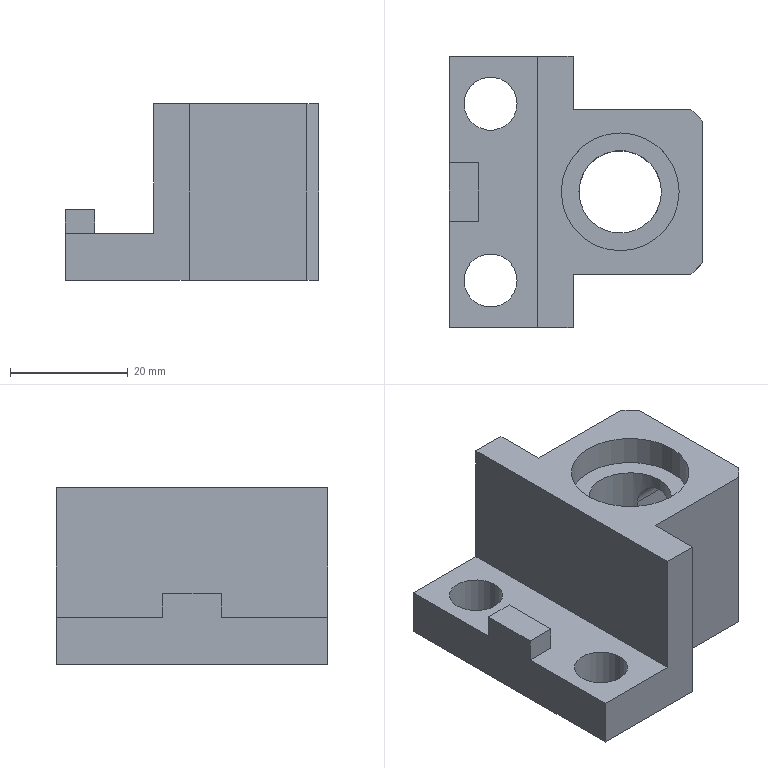Part | SolidWorks | features ICE 4, Chamfer 1, Extrusion 1 | 1 solid | 32 faces | box 43 x 46 x 30 mm | volume 25082 mm3 | plane 21 | cylinder 11 | commonest cylinder face diameters 9 x4 8 x3 14 x2 20 x2
STEP:
#1=CARTESIAN_POINT('',(13.245,4.,11.));
#2=VERTEX_POINT('',#1);
#3=CARTESIAN_POINT('',(14.5,0.,7.));
#4=VERTEX_POINT('',#3);
#5=CARTESIAN_POINT('',(13.245,4.,11.));
#6=CARTESIAN_POINT('',(13.245,4.,10.729));
#7=CARTESIAN_POINT('',(13.264,3.973,10.464));
#8=CARTESIAN_POINT('',(13.335,3.867,9.944));
#9=CARTESIAN_POINT('',(13.388,3.788,9.688));
#10=CARTESIAN_POINT('',(13.576,3.484,8.968));
#11=CARTESIAN_POINT('',(13.743,3.191,8.535));
#12=CARTESIAN_POINT('',(13.982,2.65,7.993));
#13=CARTESIAN_POINT('',(14.061,2.449,7.827));
#14=CARTESIAN_POINT('',(14.206,2.021,7.538));
#15=CARTESIAN_POINT('',(14.271,1.794,7.415));
#16=CARTESIAN_POINT('',(14.38,1.312,7.212));
#17=CARTESIAN_POINT('',(14.425,1.054,7.132));
#18=CARTESIAN_POINT('',(14.485,0.5336,7.027));
#19=CARTESIAN_POINT('',(14.5,0.269,7.));
#20=CARTESIAN_POINT('',(14.5,0.,7.));
#21=B_SPLINE_CURVE_WITH_KNOTS('',3,(#5,#6,#7,#8,#9,#10,#11,#12,#13,#14,#15,#16,#17,#18,#19,#20),.UNSPECIFIED.,.F.,.F.,(4,2,2,2,2,2,2,4),(0.,0.0008004,0.001601,0.003201,0.004002,0.004802,0.005603,0.006403),.UNSPECIFIED.);
#22=EDGE_CURVE('',#2,#4,#21,.T.);
#23=ORIENTED_EDGE('',*,*,#22,.T.);
#24=CARTESIAN_POINT('',(21.5,0.,7.));
#25=VERTEX_POINT('',#24);
#26=CARTESIAN_POINT('',(9.5,0.,7.));
#27=DIRECTION('',(1.,0.,0.));
#28=VECTOR('',#27,1000.);
#29=LINE('',#26,#28);
#30=EDGE_CURVE('',#4,#25,#29,.T.);
#31=ORIENTED_EDGE('',*,*,#30,.T.);
#32=CARTESIAN_POINT('',(21.5,4.,11.));
#33=VERTEX_POINT('',#32);
#34=CARTESIAN_POINT('',(21.5,0.,11.));
#35=DIRECTION('',(1.,0.,0.));
#36=DIRECTION('',(0.,0.,1.));
#37=AXIS2_PLACEMENT_3D('',#34,#35,#36);
#38=CIRCLE('',#37,4.);
#39=EDGE_CURVE('',#25,#33,#38,.T.);
#40=ORIENTED_EDGE('',*,*,#39,.T.);
#41=CARTESIAN_POINT('',(9.5,4.,11.));
#42=DIRECTION('',(1.,0.,0.));
#43=VECTOR('',#42,1000.);
#44=LINE('',#41,#43);
#45=EDGE_CURVE('',#2,#33,#44,.T.);
#46=ORIENTED_EDGE('',*,*,#45,.F.);
#47=EDGE_LOOP('',(#23,#31,#40,#46));
#48=FACE_OUTER_BOUND('',#47,.T.);
#49=CARTESIAN_POINT('',(9.5,0.,11.));
#50=DIRECTION('',(1.,0.,0.));
#51=DIRECTION('',(0.,0.,-1.));
#52=AXIS2_PLACEMENT_3D('',#49,#50,#51);
#53=CYLINDRICAL_SURFACE('',#52,4.);
#54=ADVANCED_FACE('',(#48),#53,.F.);
#55=CARTESIAN_POINT('',(-2.5,0.,25.));
#56=VERTEX_POINT('',#55);
#57=CARTESIAN_POINT('',(17.5,0.,25.));
#58=VERTEX_POINT('',#57);
#59=CARTESIAN_POINT('',(7.5,0.,25.));
#60=DIRECTION('',(0.,0.,1.));
#61=DIRECTION('',(1.,0.,0.));
#62=AXIS2_PLACEMENT_3D('',#59,#60,#61);
#63=CIRCLE('',#62,10.);
#64=EDGE_CURVE('',#56,#58,#63,.T.);
#65=ORIENTED_EDGE('',*,*,#64,.F.);
#66=CARTESIAN_POINT('',(-2.5,0.,30.));
#67=VERTEX_POINT('',#66);
#68=CARTESIAN_POINT('',(-2.5,0.,25.));
#69=DIRECTION('',(0.,0.,1.));
#70=VECTOR('',#69,1000.);
#71=LINE('',#68,#70);
#72=EDGE_CURVE('',#56,#67,#71,.T.);
#73=ORIENTED_EDGE('',*,*,#72,.T.);
#74=CARTESIAN_POINT('',(17.5,0.,30.));
#75=VERTEX_POINT('',#74);
#76=CARTESIAN_POINT('',(7.5,0.,30.));
#77=DIRECTION('',(0.,0.,1.));
#78=DIRECTION('',(1.,0.,0.));
#79=AXIS2_PLACEMENT_3D('',#76,#77,#78);
#80=CIRCLE('',#79,10.);
#81=EDGE_CURVE('',#67,#75,#80,.T.);
#82=ORIENTED_EDGE('',*,*,#81,.T.);
#83=CARTESIAN_POINT('',(17.5,0.,25.));
#84=DIRECTION('',(0.,0.,1.));
#85=VECTOR('',#84,1000.);
#86=LINE('',#83,#85);
#87=EDGE_CURVE('',#58,#75,#86,.T.);
#88=ORIENTED_EDGE('',*,*,#87,.F.);
#89=EDGE_LOOP('',(#65,#73,#82,#88));
#90=FACE_OUTER_BOUND('',#89,.T.);
#91=CARTESIAN_POINT('',(7.5,0.,25.));
#92=DIRECTION('',(0.,0.,1.));
#93=DIRECTION('',(1.,0.,0.));
#94=AXIS2_PLACEMENT_3D('',#91,#92,#93);
#95=CYLINDRICAL_SURFACE('',#94,10.);
#96=ADVANCED_FACE('',(#90),#95,.F.);
#97=CARTESIAN_POINT('',(-10.,-15.,8.));
#98=VERTEX_POINT('',#97);
#99=CARTESIAN_POINT('',(-19.,-15.,8.));
#100=VERTEX_POINT('',#99);
#101=CARTESIAN_POINT('',(-14.5,-15.,8.));
#102=DIRECTION('',(0.,0.,-1.));
#103=DIRECTION('',(-1.,0.,0.));
#104=AXIS2_PLACEMENT_3D('',#101,#102,#103);
#105=CIRCLE('',#104,4.5);
#106=EDGE_CURVE('',#98,#100,#105,.T.);
#107=ORIENTED_EDGE('',*,*,#106,.F.);
#108=CARTESIAN_POINT('',(-10.,-15.,0.));
#109=VERTEX_POINT('',#108);
#110=CARTESIAN_POINT('',(-10.,-15.,30.));
#111=DIRECTION('',(0.,0.,-1.));
#112=VECTOR('',#111,1000.);
#113=LINE('',#110,#112);
#114=EDGE_CURVE('',#98,#109,#113,.T.);
#115=ORIENTED_EDGE('',*,*,#114,.T.);
#116=CARTESIAN_POINT('',(-19.,-15.,0.));
#117=VERTEX_POINT('',#116);
#118=CARTESIAN_POINT('',(-14.5,-15.,0.));
#119=DIRECTION('',(0.,0.,1.));
#120=DIRECTION('',(1.,0.,0.));
#121=AXIS2_PLACEMENT_3D('',#118,#119,#120);
#122=CIRCLE('',#121,4.5);
#123=EDGE_CURVE('',#117,#109,#122,.T.);
#124=ORIENTED_EDGE('',*,*,#123,.F.);
#125=CARTESIAN_POINT('',(-19.,-15.,30.));
#126=DIRECTION('',(0.,0.,-1.));
#127=VECTOR('',#126,1000.);
#128=LINE('',#125,#127);
#129=EDGE_CURVE('',#100,#117,#128,.T.);
#130=ORIENTED_EDGE('',*,*,#129,.F.);
#131=EDGE_LOOP('',(#107,#115,#124,#130));
#132=FACE_OUTER_BOUND('',#131,.T.);
#133=CARTESIAN_POINT('',(-14.5,-15.,30.));
#134=DIRECTION('',(0.,0.,-1.));
#135=DIRECTION('',(-1.,0.,0.));
#136=AXIS2_PLACEMENT_3D('',#133,#134,#135);
#137=CYLINDRICAL_SURFACE('',#136,4.5);
#138=ADVANCED_FACE('',(#132),#137,.F.);
#139=CARTESIAN_POINT('',(-10.,15.,8.));
#140=VERTEX_POINT('',#139);
#141=CARTESIAN_POINT('',(-19.,15.,8.));
#142=VERTEX_POINT('',#141);
#143=CARTESIAN_POINT('',(-14.5,15.,8.));
#144=DIRECTION('',(0.,0.,-1.));
#145=DIRECTION('',(-1.,0.,0.));
#146=AXIS2_PLACEMENT_3D('',#143,#144,#145);
#147=CIRCLE('',#146,4.5);
#148=EDGE_CURVE('',#140,#142,#147,.T.);
#149=ORIENTED_EDGE('',*,*,#148,.F.);
#150=CARTESIAN_POINT('',(-10.,15.,0.));
#151=VERTEX_POINT('',#150);
#152=CARTESIAN_POINT('',(-10.,15.,30.));
#153=DIRECTION('',(0.,0.,-1.));
#154=VECTOR('',#153,1000.);
#155=LINE('',#152,#154);
#156=EDGE_CURVE('',#140,#151,#155,.T.);
#157=ORIENTED_EDGE('',*,*,#156,.T.);
#158=CARTESIAN_POINT('',(-19.,15.,0.));
#159=VERTEX_POINT('',#158);
#160=CARTESIAN_POINT('',(-14.5,15.,0.));
#161=DIRECTION('',(0.,0.,1.));
#162=DIRECTION('',(1.,0.,0.));
#163=AXIS2_PLACEMENT_3D('',#160,#161,#162);
#164=CIRCLE('',#163,4.5);
#165=EDGE_CURVE('',#159,#151,#164,.T.);
#166=ORIENTED_EDGE('',*,*,#165,.F.);
#167=CARTESIAN_POINT('',(-19.,15.,30.));
#168=DIRECTION('',(0.,0.,-1.));
#169=VECTOR('',#168,1000.);
#170=LINE('',#167,#169);
#171=EDGE_CURVE('',#142,#159,#170,.T.);
#172=ORIENTED_EDGE('',*,*,#171,.F.);
#173=EDGE_LOOP('',(#149,#157,#166,#172));
#174=FACE_OUTER_BOUND('',#173,.T.);
#175=CARTESIAN_POINT('',(-14.5,15.,30.));
#176=DIRECTION('',(0.,0.,-1.));
#177=DIRECTION('',(-1.,0.,0.));
#178=AXIS2_PLACEMENT_3D('',#175,#176,#177);
#179=CYLINDRICAL_SURFACE('',#178,4.5);
#180=ADVANCED_FACE('',(#174),#179,.F.);
#181=CARTESIAN_POINT('',(0.5,0.,25.));
#182=VERTEX_POINT('',#181);
#183=CARTESIAN_POINT('',(14.5,0.,25.));
#184=VERTEX_POINT('',#183);
#185=CARTESIAN_POINT('',(7.5,0.,25.));
#186=DIRECTION('',(0.,0.,1.));
#187=DIRECTION('',(1.,0.,0.));
#188=AXIS2_PLACEMENT_3D('',#185,#186,#187);
#189=CIRCLE('',#188,7.);
#190=EDGE_CURVE('',#182,#184,#189,.T.);
#191=ORIENTED_EDGE('',*,*,#190,.T.);
#192=CARTESIAN_POINT('',(14.5,0.,23.));
#193=VERTEX_POINT('',#192);
#194=CARTESIAN_POINT('',(14.5,0.,30.));
#195=DIRECTION('',(0.,0.,-1.));
#196=VECTOR('',#195,1000.);
#197=LINE('',#194,#196);
#198=EDGE_CURVE('',#184,#193,#197,.T.);
#199=ORIENTED_EDGE('',*,*,#198,.T.);
#200=CARTESIAN_POINT('',(13.245,-4.,19.));
#201=VERTEX_POINT('',#200);
#202=CARTESIAN_POINT('',(13.245,-4.,19.));
#203=CARTESIAN_POINT('',(13.245,-4.,19.271));
#204=CARTESIAN_POINT('',(13.264,-3.973,19.536));
#205=CARTESIAN_POINT('',(13.335,-3.867,20.056));
#206=CARTESIAN_POINT('',(13.388,-3.788,20.312));
#207=CARTESIAN_POINT('',(13.576,-3.484,21.032));
#208=CARTESIAN_POINT('',(13.743,-3.191,21.465));
#209=CARTESIAN_POINT('',(13.982,-2.65,22.007));
#210=CARTESIAN_POINT('',(14.061,-2.449,22.173));
#211=CARTESIAN_POINT('',(14.206,-2.021,22.462));
#212=CARTESIAN_POINT('',(14.271,-1.794,22.585));
#213=CARTESIAN_POINT('',(14.38,-1.312,22.788));
#214=CARTESIAN_POINT('',(14.425,-1.054,22.868));
#215=CARTESIAN_POINT('',(14.485,-0.5336,22.973));
#216=CARTESIAN_POINT('',(14.5,-0.269,23.));
#217=CARTESIAN_POINT('',(14.5,0.,23.));
#218=B_SPLINE_CURVE_WITH_KNOTS('',3,(#202,#203,#204,#205,#206,#207,#208,#209,#210,#211,#212,#213,#214,#215,#216,#217),.UNSPECIFIED.,.F.,.F.,(4,2,2,2,2,2,2,4),(0.,0.0008004,0.001601,0.003201,0.004002,0.004802,0.005603,0.006403),.UNSPECIFIED.);
#219=EDGE_CURVE('',#201,#193,#218,.T.);
#220=ORIENTED_EDGE('',*,*,#219,.F.);
#221=CARTESIAN_POINT('',(13.245,-4.,11.));
#222=VERTEX_POINT('',#221);
#223=CARTESIAN_POINT('',(13.245,-4.,30.));
#224=DIRECTION('',(0.,0.,1.));
#225=VECTOR('',#224,1000.);
#226=LINE('',#223,#225);
#227=EDGE_CURVE('',#222,#201,#226,.T.);
#228=ORIENTED_EDGE('',*,*,#227,.F.);
#229=CARTESIAN_POINT('',(14.5,0.,7.));
#230=CARTESIAN_POINT('',(14.5,-0.1342,7.));
#231=CARTESIAN_POINT('',(14.496,-0.27,7.007));
#232=CARTESIAN_POINT('',(14.481,-0.5365,7.034));
#233=CARTESIAN_POINT('',(14.469,-0.668,7.054));
#234=CARTESIAN_POINT('',(14.425,-1.058,7.133));
#235=CARTESIAN_POINT('',(14.38,-1.314,7.213));
#236=CARTESIAN_POINT('',(14.27,-1.798,7.417));
#237=CARTESIAN_POINT('',(14.204,-2.026,7.541));
#238=CARTESIAN_POINT('',(14.059,-2.455,7.831));
#239=CARTESIAN_POINT('',(13.98,-2.654,7.996));
#240=CARTESIAN_POINT('',(13.821,-3.014,8.358));
#241=CARTESIAN_POINT('',(13.74,-3.177,8.556));
#242=CARTESIAN_POINT('',(13.585,-3.464,8.984));
#243=CARTESIAN_POINT('',(13.513,-3.586,9.21));
#244=CARTESIAN_POINT('',(13.388,-3.787,9.687));
#245=CARTESIAN_POINT('',(13.336,-3.867,9.942));
#246=CARTESIAN_POINT('',(13.264,-3.973,10.463));
#247=CARTESIAN_POINT('',(13.245,-4.,10.729));
#248=CARTESIAN_POINT('',(13.245,-4.,11.));
#249=B_SPLINE_CURVE_WITH_KNOTS('',3,(#229,#230,#231,#232,#233,#234,#235,#236,#237,#238,#239,#240,#241,#242,#243,#244,#245,#246,#247,#248),.UNSPECIFIED.,.F.,.F.,(4,2,2,2,2,2,2,2,2,4),(0.006403,0.006802,0.007202,0.008,0.008799,0.009597,0.0104,0.01119,0.01199,0.01279),.UNSPECIFIED.);
#250=EDGE_CURVE('',#4,#222,#249,.T.);
#251=ORIENTED_EDGE('',*,*,#250,.F.);
#252=CARTESIAN_POINT('',(14.5,0.,0.));
#253=VERTEX_POINT('',#252);
#254=CARTESIAN_POINT('',(14.5,0.,30.));
#255=DIRECTION('',(0.,0.,-1.));
#256=VECTOR('',#255,1000.);
#257=LINE('',#254,#256);
#258=EDGE_CURVE('',#4,#253,#257,.T.);
#259=ORIENTED_EDGE('',*,*,#258,.T.);
#260=CARTESIAN_POINT('',(0.5,0.,0.));
#261=VERTEX_POINT('',#260);
#262=CARTESIAN_POINT('',(7.5,0.,0.));
#263=DIRECTION('',(0.,0.,1.));
#264=DIRECTION('',(1.,0.,0.));
#265=AXIS2_PLACEMENT_3D('',#262,#263,#264);
#266=CIRCLE('',#265,7.);
#267=EDGE_CURVE('',#261,#253,#266,.T.);
#268=ORIENTED_EDGE('',*,*,#267,.F.);
#269=CARTESIAN_POINT('',(0.5,0.,30.));
#270=DIRECTION('',(0.,0.,-1.));
#271=VECTOR('',#270,1000.);
#272=LINE('',#269,#271);
#273=EDGE_CURVE('',#182,#261,#272,.T.);
#274=ORIENTED_EDGE('',*,*,#273,.F.);
#275=EDGE_LOOP('',(#191,#199,#220,#228,#251,#259,#268,#274));
#276=FACE_OUTER_BOUND('',#275,.T.);
#277=CARTESIAN_POINT('',(7.5,0.,30.));
#278=DIRECTION('',(0.,0.,-1.));
#279=DIRECTION('',(-1.,0.,0.));
#280=AXIS2_PLACEMENT_3D('',#277,#278,#279);
#281=CYLINDRICAL_SURFACE('',#280,7.);
#282=ADVANCED_FACE('',(#276),#281,.F.);
#283=CARTESIAN_POINT('',(-14.5,-15.,8.));
#284=DIRECTION('',(0.,0.,-1.));
#285=DIRECTION('',(-1.,0.,0.));
#286=AXIS2_PLACEMENT_3D('',#283,#284,#285);
#287=CIRCLE('',#286,4.5);
#288=EDGE_CURVE('',#100,#98,#287,.T.);
#289=ORIENTED_EDGE('',*,*,#288,.T.);
#290=ORIENTED_EDGE('',*,*,#106,.T.);
#291=EDGE_LOOP('',(#289,#290));
#292=FACE_BOUND('',#291,.T.);
#293=CARTESIAN_POINT('',(-14.5,15.,8.));
#294=DIRECTION('',(0.,0.,-1.));
#295=DIRECTION('',(-1.,0.,0.));
#296=AXIS2_PLACEMENT_3D('',#293,#294,#295);
#297=CIRCLE('',#296,4.5);
#298=EDGE_CURVE('',#142,#140,#297,.T.);
#299=ORIENTED_EDGE('',*,*,#298,.T.);
#300=ORIENTED_EDGE('',*,*,#148,.T.);
#301=EDGE_LOOP('',(#299,#300));
#302=FACE_BOUND('',#301,.T.);
#303=CARTESIAN_POINT('',(-21.5,-5.,8.));
#304=VERTEX_POINT('',#303);
#305=CARTESIAN_POINT('',(-16.5,-5.,8.));
#306=VERTEX_POINT('',#305);
#307=CARTESIAN_POINT('',(-16.5,-5.,8.));
#308=DIRECTION('',(1.,0.,0.));
#309=VECTOR('',#308,1000.);
#310=LINE('',#307,#309);
#311=EDGE_CURVE('',#304,#306,#310,.T.);
#312=ORIENTED_EDGE('',*,*,#311,.F.);
#313=CARTESIAN_POINT('',(-21.5,-23.,8.));
#314=VERTEX_POINT('',#313);
#315=CARTESIAN_POINT('',(-21.5,-23.,8.));
#316=DIRECTION('',(0.,1.,0.));
#317=VECTOR('',#316,1000.);
#318=LINE('',#315,#317);
#319=EDGE_CURVE('',#314,#304,#318,.T.);
#320=ORIENTED_EDGE('',*,*,#319,.F.);
#321=CARTESIAN_POINT('',(-6.5,-23.,8.));
#322=VERTEX_POINT('',#321);
#323=CARTESIAN_POINT('',(-6.5,-23.,8.));
#324=DIRECTION('',(-1.,0.,0.));
#325=VECTOR('',#324,1000.);
#326=LINE('',#323,#325);
#327=EDGE_CURVE('',#322,#314,#326,.T.);
#328=ORIENTED_EDGE('',*,*,#327,.F.);
#329=CARTESIAN_POINT('',(-6.5,23.,8.));
#330=VERTEX_POINT('',#329);
#331=CARTESIAN_POINT('',(-6.5,-23.,8.));
#332=DIRECTION('',(0.,1.,0.));
#333=VECTOR('',#332,1000.);
#334=LINE('',#331,#333);
#335=EDGE_CURVE('',#322,#330,#334,.T.);
#336=ORIENTED_EDGE('',*,*,#335,.T.);
#337=CARTESIAN_POINT('',(-21.5,23.,8.));
#338=VERTEX_POINT('',#337);
#339=CARTESIAN_POINT('',(-6.5,23.,8.));
#340=DIRECTION('',(-1.,0.,0.));
#341=VECTOR('',#340,1000.);
#342=LINE('',#339,#341);
#343=EDGE_CURVE('',#330,#338,#342,.T.);
#344=ORIENTED_EDGE('',*,*,#343,.T.);
#345=CARTESIAN_POINT('',(-21.5,5.,8.));
#346=VERTEX_POINT('',#345);
#347=CARTESIAN_POINT('',(-21.5,-23.,8.));
#348=DIRECTION('',(0.,1.,0.));
#349=VECTOR('',#348,1000.);
#350=LINE('',#347,#349);
#351=EDGE_CURVE('',#346,#338,#350,.T.);
#352=ORIENTED_EDGE('',*,*,#351,.F.);
#353=CARTESIAN_POINT('',(-16.5,5.,8.));
#354=VERTEX_POINT('',#353);
#355=CARTESIAN_POINT('',(-16.5,5.,8.));
#356=DIRECTION('',(-1.,0.,0.));
#357=VECTOR('',#356,1000.);
#358=LINE('',#355,#357);
#359=EDGE_CURVE('',#354,#346,#358,.T.);
#360=ORIENTED_EDGE('',*,*,#359,.F.);
#361=CARTESIAN_POINT('',(-16.5,-5.,8.));
#362=DIRECTION('',(0.,1.,0.));
#363=VECTOR('',#362,1000.);
#364=LINE('',#361,#363);
#365=EDGE_CURVE('',#306,#354,#364,.T.);
#366=ORIENTED_EDGE('',*,*,#365,.F.);
#367=EDGE_LOOP('',(#312,#320,#328,#336,#344,#352,#360,#366));
#368=FACE_OUTER_BOUND('',#367,.T.);
#369=CARTESIAN_POINT('',(-6.5,-23.,8.));
#370=DIRECTION('',(0.,0.,-1.));
#371=DIRECTION('',(-1.,0.,0.));
#372=AXIS2_PLACEMENT_3D('',#369,#370,#371);
#373=PLANE('',#372);
#374=ADVANCED_FACE('',(#292,#302,#368),#373,.F.);
#375=ORIENTED_EDGE('',*,*,#198,.F.);
#376=CARTESIAN_POINT('',(7.5,0.,25.));
#377=DIRECTION('',(0.,0.,1.));
#378=DIRECTION('',(1.,0.,0.));
#379=AXIS2_PLACEMENT_3D('',#376,#377,#378);
#380=CIRCLE('',#379,7.);
#381=EDGE_CURVE('',#184,#182,#380,.T.);
#382=ORIENTED_EDGE('',*,*,#381,.T.);
#383=ORIENTED_EDGE('',*,*,#273,.T.);
#384=CARTESIAN_POINT('',(7.5,0.,0.));
#385=DIRECTION('',(0.,0.,1.));
#386=DIRECTION('',(1.,0.,0.));
#387=AXIS2_PLACEMENT_3D('',#384,#385,#386);
#388=CIRCLE('',#387,7.);
#389=EDGE_CURVE('',#253,#261,#388,.T.);
#390=ORIENTED_EDGE('',*,*,#389,.F.);
#391=ORIENTED_EDGE('',*,*,#258,.F.);
#392=ORIENTED_EDGE('',*,*,#22,.F.);
#393=CARTESIAN_POINT('',(13.245,4.,19.));
#394=VERTEX_POINT('',#393);
#395=CARTESIAN_POINT('',(13.245,4.,30.));
#396=DIRECTION('',(0.,0.,-1.));
#397=VECTOR('',#396,1000.);
#398=LINE('',#395,#397);
#399=EDGE_CURVE('',#394,#2,#398,.T.);
#400=ORIENTED_EDGE('',*,*,#399,.F.);
#401=CARTESIAN_POINT('',(14.5,0.,23.));
#402=CARTESIAN_POINT('',(14.5,0.1342,23.));
#403=CARTESIAN_POINT('',(14.496,0.27,22.993));
#404=CARTESIAN_POINT('',(14.481,0.5365,22.966));
#405=CARTESIAN_POINT('',(14.469,0.668,22.946));
#406=CARTESIAN_POINT('',(14.425,1.058,22.867));
#407=CARTESIAN_POINT('',(14.38,1.314,22.787));
#408=CARTESIAN_POINT('',(14.27,1.798,22.583));
#409=CARTESIAN_POINT('',(14.204,2.026,22.459));
#410=CARTESIAN_POINT('',(14.059,2.455,22.169));
#411=CARTESIAN_POINT('',(13.98,2.654,22.004));
#412=CARTESIAN_POINT('',(13.821,3.014,21.642));
#413=CARTESIAN_POINT('',(13.74,3.177,21.444));
#414=CARTESIAN_POINT('',(13.585,3.464,21.016));
#415=CARTESIAN_POINT('',(13.513,3.586,20.79));
#416=CARTESIAN_POINT('',(13.388,3.787,20.313));
#417=CARTESIAN_POINT('',(13.336,3.867,20.058));
#418=CARTESIAN_POINT('',(13.264,3.973,19.537));
#419=CARTESIAN_POINT('',(13.245,4.,19.271));
#420=CARTESIAN_POINT('',(13.245,4.,19.));
#421=B_SPLINE_CURVE_WITH_KNOTS('',3,(#401,#402,#403,#404,#405,#406,#407,#408,#409,#410,#411,#412,#413,#414,#415,#416,#417,#418,#419,#420),.UNSPECIFIED.,.F.,.F.,(4,2,2,2,2,2,2,2,2,4),(0.006403,0.006802,0.007202,0.008,0.008799,0.009597,0.0104,0.01119,0.01199,0.01279),.UNSPECIFIED.);
#422=EDGE_CURVE('',#193,#394,#421,.T.);
#423=ORIENTED_EDGE('',*,*,#422,.F.);
#424=EDGE_LOOP('',(#375,#382,#383,#390,#391,#392,#400,#423));
#425=FACE_OUTER_BOUND('',#424,.T.);
#426=CARTESIAN_POINT('',(7.5,0.,30.));
#427=DIRECTION('',(0.,0.,-1.));
#428=DIRECTION('',(-1.,0.,0.));
#429=AXIS2_PLACEMENT_3D('',#426,#427,#428);
#430=CYLINDRICAL_SURFACE('',#429,7.);
#431=ADVANCED_FACE('',(#425),#430,.F.);
#432=CARTESIAN_POINT('',(7.5,0.,30.));
#433=DIRECTION('',(0.,0.,1.));
#434=DIRECTION('',(1.,0.,0.));
#435=AXIS2_PLACEMENT_3D('',#432,#433,#434);
#436=CIRCLE('',#435,10.);
#437=EDGE_CURVE('',#75,#67,#436,.T.);
#438=ORIENTED_EDGE('',*,*,#437,.F.);
#439=ORIENTED_EDGE('',*,*,#81,.F.);
#440=EDGE_LOOP('',(#438,#439));
#441=FACE_BOUND('',#440,.T.);
#442=CARTESIAN_POINT('',(-0.5,-14.,30.));
#443=VERTEX_POINT('',#442);
#444=CARTESIAN_POINT('',(19.5,-14.,30.));
#445=VERTEX_POINT('',#444);
#446=CARTESIAN_POINT('',(-0.5,-14.,30.));
#447=DIRECTION('',(1.,0.,0.));
#448=VECTOR('',#447,1000.);
#449=LINE('',#446,#448);
#450=EDGE_CURVE('',#443,#445,#449,.T.);
#451=ORIENTED_EDGE('',*,*,#450,.T.);
#452=CARTESIAN_POINT('',(21.5,-12.,30.));
#453=VERTEX_POINT('',#452);
#454=CARTESIAN_POINT('',(16.75,-16.75,30.));
#455=DIRECTION('',(0.7071,0.7071,0.));
#456=VECTOR('',#455,1000.);
#457=LINE('',#454,#456);
#458=EDGE_CURVE('',#445,#453,#457,.T.);
#459=ORIENTED_EDGE('',*,*,#458,.T.);
#460=CARTESIAN_POINT('',(21.5,12.,30.));
#461=VERTEX_POINT('',#460);
#462=CARTESIAN_POINT('',(21.5,14.,30.));
#463=DIRECTION('',(0.,1.,0.));
#464=VECTOR('',#463,1000.);
#465=LINE('',#462,#464);
#466=EDGE_CURVE('',#453,#461,#465,.T.);
#467=ORIENTED_EDGE('',*,*,#466,.T.);
#468=CARTESIAN_POINT('',(19.5,14.,30.));
#469=VERTEX_POINT('',#468);
#470=CARTESIAN_POINT('',(16.75,16.75,30.));
#471=DIRECTION('',(-0.7071,0.7071,0.));
#472=VECTOR('',#471,1000.);
#473=LINE('',#470,#472);
#474=EDGE_CURVE('',#461,#469,#473,.T.);
#475=ORIENTED_EDGE('',*,*,#474,.T.);
#476=CARTESIAN_POINT('',(-0.5,14.,30.));
#477=VERTEX_POINT('',#476);
#478=CARTESIAN_POINT('',(-0.5,14.,30.));
#479=DIRECTION('',(-1.,0.,0.));
#480=VECTOR('',#479,1000.);
#481=LINE('',#478,#480);
#482=EDGE_CURVE('',#469,#477,#481,.T.);
#483=ORIENTED_EDGE('',*,*,#482,.T.);
#484=CARTESIAN_POINT('',(-0.5,23.,30.));
#485=VERTEX_POINT('',#484);
#486=CARTESIAN_POINT('',(-0.5,23.,30.));
#487=DIRECTION('',(0.,1.,0.));
#488=VECTOR('',#487,1000.);
#489=LINE('',#486,#488);
#490=EDGE_CURVE('',#477,#485,#489,.T.);
#491=ORIENTED_EDGE('',*,*,#490,.T.);
#492=CARTESIAN_POINT('',(-6.5,23.,30.));
#493=VERTEX_POINT('',#492);
#494=CARTESIAN_POINT('',(-21.5,23.,30.));
#495=DIRECTION('',(-1.,0.,0.));
#496=VECTOR('',#495,1000.);
#497=LINE('',#494,#496);
#498=EDGE_CURVE('',#485,#493,#497,.T.);
#499=ORIENTED_EDGE('',*,*,#498,.T.);
#500=CARTESIAN_POINT('',(-6.5,-23.,30.));
#501=VERTEX_POINT('',#500);
#502=CARTESIAN_POINT('',(-6.5,-23.,30.));
#503=DIRECTION('',(0.,1.,0.));
#504=VECTOR('',#503,1000.);
#505=LINE('',#502,#504);
#506=EDGE_CURVE('',#501,#493,#505,.T.);
#507=ORIENTED_EDGE('',*,*,#506,.F.);
#508=CARTESIAN_POINT('',(-0.5,-23.,30.));
#509=VERTEX_POINT('',#508);
#510=CARTESIAN_POINT('',(-21.5,-23.,30.));
#511=DIRECTION('',(1.,0.,0.));
#512=VECTOR('',#511,1000.);
#513=LINE('',#510,#512);
#514=EDGE_CURVE('',#501,#509,#513,.T.);
#515=ORIENTED_EDGE('',*,*,#514,.T.);
#516=CARTESIAN_POINT('',(-0.5,-14.,30.));
#517=DIRECTION('',(0.,1.,0.));
#518=VECTOR('',#517,1000.);
#519=LINE('',#516,#518);
#520=EDGE_CURVE('',#509,#443,#519,.T.);
#521=ORIENTED_EDGE('',*,*,#520,.T.);
#522=EDGE_LOOP('',(#451,#459,#467,#475,#483,#491,#499,#507,#515,#521));
#523=FACE_OUTER_BOUND('',#522,.T.);
#524=CARTESIAN_POINT('',(0.,0.,30.));
#525=DIRECTION('',(0.,0.,1.));
#526=DIRECTION('',(1.,0.,0.));
#527=AXIS2_PLACEMENT_3D('',#524,#525,#526);
#528=PLANE('',#527);
#529=ADVANCED_FACE('',(#441,#523),#528,.T.);
#530=ORIENTED_EDGE('',*,*,#165,.T.);
#531=CARTESIAN_POINT('',(-14.5,15.,0.));
#532=DIRECTION('',(0.,0.,1.));
#533=DIRECTION('',(1.,0.,0.));
#534=AXIS2_PLACEMENT_3D('',#531,#532,#533);
#535=CIRCLE('',#534,4.5);
#536=EDGE_CURVE('',#151,#159,#535,.T.);
#537=ORIENTED_EDGE('',*,*,#536,.T.);
#538=EDGE_LOOP('',(#530,#537));
#539=FACE_BOUND('',#538,.T.);
#540=CARTESIAN_POINT('',(21.5,-12.,0.));
#541=VERTEX_POINT('',#540);
#542=CARTESIAN_POINT('',(21.5,12.,0.));
#543=VERTEX_POINT('',#542);
#544=CARTESIAN_POINT('',(21.5,14.,0.));
#545=DIRECTION('',(0.,1.,0.));
#546=VECTOR('',#545,1000.);
#547=LINE('',#544,#546);
#548=EDGE_CURVE('',#541,#543,#547,.T.);
#549=ORIENTED_EDGE('',*,*,#548,.F.);
#550=CARTESIAN_POINT('',(19.5,-14.,0.));
#551=VERTEX_POINT('',#550);
#552=CARTESIAN_POINT('',(21.5,-12.,0.));
#553=DIRECTION('',(-0.7071,-0.7071,0.));
#554=VECTOR('',#553,1000.);
#555=LINE('',#552,#554);
#556=EDGE_CURVE('',#541,#551,#555,.T.);
#557=ORIENTED_EDGE('',*,*,#556,.T.);
#558=CARTESIAN_POINT('',(-0.5,-14.,0.));
#559=VERTEX_POINT('',#558);
#560=CARTESIAN_POINT('',(-0.5,-14.,0.));
#561=DIRECTION('',(1.,0.,0.));
#562=VECTOR('',#561,1000.);
#563=LINE('',#560,#562);
#564=EDGE_CURVE('',#559,#551,#563,.T.);
#565=ORIENTED_EDGE('',*,*,#564,.F.);
#566=CARTESIAN_POINT('',(-0.5,-23.,0.));
#567=VERTEX_POINT('',#566);
#568=CARTESIAN_POINT('',(-0.5,-14.,0.));
#569=DIRECTION('',(0.,1.,0.));
#570=VECTOR('',#569,1000.);
#571=LINE('',#568,#570);
#572=EDGE_CURVE('',#567,#559,#571,.T.);
#573=ORIENTED_EDGE('',*,*,#572,.F.);
#574=CARTESIAN_POINT('',(-21.5,-23.,0.));
#575=VERTEX_POINT('',#574);
#576=CARTESIAN_POINT('',(-21.5,-23.,0.));
#577=DIRECTION('',(1.,0.,0.));
#578=VECTOR('',#577,1000.);
#579=LINE('',#576,#578);
#580=EDGE_CURVE('',#575,#567,#579,.T.);
#581=ORIENTED_EDGE('',*,*,#580,.F.);
#582=CARTESIAN_POINT('',(-21.5,23.,0.));
#583=VERTEX_POINT('',#582);
#584=CARTESIAN_POINT('',(-21.5,23.,0.));
#585=DIRECTION('',(0.,-1.,0.));
#586=VECTOR('',#585,1000.);
#587=LINE('',#584,#586);
#588=EDGE_CURVE('',#583,#575,#587,.T.);
#589=ORIENTED_EDGE('',*,*,#588,.F.);
#590=CARTESIAN_POINT('',(-0.5,23.,0.));
#591=VERTEX_POINT('',#590);
#592=CARTESIAN_POINT('',(-21.5,23.,0.));
#593=DIRECTION('',(-1.,0.,0.));
#594=VECTOR('',#593,1000.);
#595=LINE('',#592,#594);
#596=EDGE_CURVE('',#591,#583,#595,.T.);
#597=ORIENTED_EDGE('',*,*,#596,.F.);
#598=CARTESIAN_POINT('',(-0.5,14.,0.));
#599=VERTEX_POINT('',#598);
#600=CARTESIAN_POINT('',(-0.5,23.,0.));
#601=DIRECTION('',(0.,1.,0.));
#602=VECTOR('',#601,1000.);
#603=LINE('',#600,#602);
#604=EDGE_CURVE('',#599,#591,#603,.T.);
#605=ORIENTED_EDGE('',*,*,#604,.F.);
#606=CARTESIAN_POINT('',(19.5,14.,0.));
#607=VERTEX_POINT('',#606);
#608=CARTESIAN_POINT('',(-0.5,14.,0.));
#609=DIRECTION('',(-1.,0.,0.));
#610=VECTOR('',#609,1000.);
#611=LINE('',#608,#610);
#612=EDGE_CURVE('',#607,#599,#611,.T.);
#613=ORIENTED_EDGE('',*,*,#612,.F.);
#614=CARTESIAN_POINT('',(19.5,14.,0.));
#615=DIRECTION('',(0.7071,-0.7071,0.));
#616=VECTOR('',#615,1000.);
#617=LINE('',#614,#616);
#618=EDGE_CURVE('',#607,#543,#617,.T.);
#619=ORIENTED_EDGE('',*,*,#618,.T.);
#620=EDGE_LOOP('',(#549,#557,#565,#573,#581,#589,#597,#605,#613,#619));
#621=FACE_OUTER_BOUND('',#620,.T.);
#622=ORIENTED_EDGE('',*,*,#267,.T.);
#623=ORIENTED_EDGE('',*,*,#389,.T.);
#624=EDGE_LOOP('',(#622,#623));
#625=FACE_BOUND('',#624,.T.);
#626=ORIENTED_EDGE('',*,*,#123,.T.);
#627=CARTESIAN_POINT('',(-14.5,-15.,0.));
#628=DIRECTION('',(0.,0.,1.));
#629=DIRECTION('',(1.,0.,0.));
#630=AXIS2_PLACEMENT_3D('',#627,#628,#629);
#631=CIRCLE('',#630,4.5);
#632=EDGE_CURVE('',#109,#117,#631,.T.);
#633=ORIENTED_EDGE('',*,*,#632,.T.);
#634=EDGE_LOOP('',(#626,#633));
#635=FACE_BOUND('',#634,.T.);
#636=CARTESIAN_POINT('',(0.,0.,0.));
#637=DIRECTION('',(0.,0.,1.));
#638=DIRECTION('',(1.,0.,0.));
#639=AXIS2_PLACEMENT_3D('',#636,#637,#638);
#640=PLANE('',#639);
#641=ADVANCED_FACE('',(#539,#621,#625,#635),#640,.F.);
#642=CARTESIAN_POINT('',(-21.5,-23.,30.));
#643=DIRECTION('',(0.,0.,-1.));
#644=VECTOR('',#643,1000.);
#645=LINE('',#642,#644);
#646=EDGE_CURVE('',#314,#575,#645,.T.);
#647=ORIENTED_EDGE('',*,*,#646,.F.);
#648=ORIENTED_EDGE('',*,*,#319,.T.);
#649=CARTESIAN_POINT('',(-21.5,-5.,12.));
#650=VERTEX_POINT('',#649);
#651=CARTESIAN_POINT('',(-21.5,-5.,12.));
#652=DIRECTION('',(0.,0.,-1.));
#653=VECTOR('',#652,1000.);
#654=LINE('',#651,#653);
#655=EDGE_CURVE('',#650,#304,#654,.T.);
#656=ORIENTED_EDGE('',*,*,#655,.F.);
#657=CARTESIAN_POINT('',(-21.5,5.,12.));
#658=VERTEX_POINT('',#657);
#659=CARTESIAN_POINT('',(-21.5,-5.,12.));
#660=DIRECTION('',(0.,-1.,0.));
#661=VECTOR('',#660,1000.);
#662=LINE('',#659,#661);
#663=EDGE_CURVE('',#658,#650,#662,.T.);
#664=ORIENTED_EDGE('',*,*,#663,.F.);
#665=CARTESIAN_POINT('',(-21.5,5.,12.));
#666=DIRECTION('',(0.,0.,-1.));
#667=VECTOR('',#666,1000.);
#668=LINE('',#665,#667);
#669=EDGE_CURVE('',#658,#346,#668,.T.);
#670=ORIENTED_EDGE('',*,*,#669,.T.);
#671=ORIENTED_EDGE('',*,*,#351,.T.);
#672=CARTESIAN_POINT('',(-21.5,23.,30.));
#673=DIRECTION('',(0.,0.,-1.));
#674=VECTOR('',#673,1000.);
#675=LINE('',#672,#674);
#676=EDGE_CURVE('',#338,#583,#675,.T.);
#677=ORIENTED_EDGE('',*,*,#676,.T.);
#678=ORIENTED_EDGE('',*,*,#588,.T.);
#679=EDGE_LOOP('',(#647,#648,#656,#664,#670,#671,#677,#678));
#680=FACE_OUTER_BOUND('',#679,.T.);
#681=CARTESIAN_POINT('',(-21.5,23.,30.));
#682=DIRECTION('',(1.,0.,0.));
#683=DIRECTION('',(0.,1.,0.));
#684=AXIS2_PLACEMENT_3D('',#681,#682,#683);
#685=PLANE('',#684);
#686=ADVANCED_FACE('',(#680),#685,.F.);
#687=CARTESIAN_POINT('',(-6.5,-23.,30.));
#688=DIRECTION('',(0.,0.,-1.));
#689=VECTOR('',#688,1000.);
#690=LINE('',#687,#689);
#691=EDGE_CURVE('',#501,#322,#690,.T.);
#692=ORIENTED_EDGE('',*,*,#691,.T.);
#693=ORIENTED_EDGE('',*,*,#327,.T.);
#694=ORIENTED_EDGE('',*,*,#646,.T.);
#695=ORIENTED_EDGE('',*,*,#580,.T.);
#696=CARTESIAN_POINT('',(-0.5,-23.,30.));
#697=DIRECTION('',(0.,0.,-1.));
#698=VECTOR('',#697,1000.);
#699=LINE('',#696,#698);
#700=EDGE_CURVE('',#509,#567,#699,.T.);
#701=ORIENTED_EDGE('',*,*,#700,.F.);
#702=ORIENTED_EDGE('',*,*,#514,.F.);
#703=EDGE_LOOP('',(#692,#693,#694,#695,#701,#702));
#704=FACE_OUTER_BOUND('',#703,.T.);
#705=CARTESIAN_POINT('',(-21.5,-23.,30.));
#706=DIRECTION('',(0.,1.,0.));
#707=DIRECTION('',(0.,0.,1.));
#708=AXIS2_PLACEMENT_3D('',#705,#706,#707);
#709=PLANE('',#708);
#710=ADVANCED_FACE('',(#704),#709,.F.);
#711=ORIENTED_EDGE('',*,*,#572,.T.);
#712=CARTESIAN_POINT('',(-0.5,-14.,30.));
#713=DIRECTION('',(0.,0.,-1.));
#714=VECTOR('',#713,1000.);
#715=LINE('',#712,#714);
#716=EDGE_CURVE('',#443,#559,#715,.T.);
#717=ORIENTED_EDGE('',*,*,#716,.F.);
#718=ORIENTED_EDGE('',*,*,#520,.F.);
#719=ORIENTED_EDGE('',*,*,#700,.T.);
#720=EDGE_LOOP('',(#711,#717,#718,#719));
#721=FACE_OUTER_BOUND('',#720,.T.);
#722=CARTESIAN_POINT('',(-0.5,-14.,30.));
#723=DIRECTION('',(-1.,0.,0.));
#724=DIRECTION('',(0.,0.,1.));
#725=AXIS2_PLACEMENT_3D('',#722,#723,#724);
#726=PLANE('',#725);
#727=ADVANCED_FACE('',(#721),#726,.F.);
#728=ORIENTED_EDGE('',*,*,#564,.T.);
#729=CARTESIAN_POINT('',(19.5,-14.,30.));
#730=DIRECTION('',(0.,0.,1.));
#731=VECTOR('',#730,1000.);
#732=LINE('',#729,#731);
#733=EDGE_CURVE('',#551,#445,#732,.T.);
#734=ORIENTED_EDGE('',*,*,#733,.T.);
#735=ORIENTED_EDGE('',*,*,#450,.F.);
#736=ORIENTED_EDGE('',*,*,#716,.T.);
#737=EDGE_LOOP('',(#728,#734,#735,#736));
#738=FACE_OUTER_BOUND('',#737,.T.);
#739=CARTESIAN_POINT('',(-0.5,-14.,30.));
#740=DIRECTION('',(0.,1.,0.));
#741=DIRECTION('',(-1.,0.,0.));
#742=AXIS2_PLACEMENT_3D('',#739,#740,#741);
#743=PLANE('',#742);
#744=ADVANCED_FACE('',(#738),#743,.F.);
#745=CARTESIAN_POINT('',(21.5,-4.,19.));
#746=VERTEX_POINT('',#745);
#747=CARTESIAN_POINT('',(21.5,-4.,11.));
#748=VERTEX_POINT('',#747);
#749=CARTESIAN_POINT('',(21.5,-4.,19.));
#750=DIRECTION('',(0.,0.,-1.));
#751=VECTOR('',#750,1000.);
#752=LINE('',#749,#751);
#753=EDGE_CURVE('',#746,#748,#752,.T.);
#754=ORIENTED_EDGE('',*,*,#753,.F.);
#755=CARTESIAN_POINT('',(21.5,4.,19.));
#756=VERTEX_POINT('',#755);
#757=CARTESIAN_POINT('',(21.5,0.,19.));
#758=DIRECTION('',(1.,0.,0.));
#759=DIRECTION('',(0.,0.,-1.));
#760=AXIS2_PLACEMENT_3D('',#757,#758,#759);
#761=CIRCLE('',#760,4.);
#762=EDGE_CURVE('',#756,#746,#761,.T.);
#763=ORIENTED_EDGE('',*,*,#762,.F.);
#764=CARTESIAN_POINT('',(21.5,4.,19.));
#765=DIRECTION('',(0.,0.,1.));
#766=VECTOR('',#765,1000.);
#767=LINE('',#764,#766);
#768=EDGE_CURVE('',#33,#756,#767,.T.);
#769=ORIENTED_EDGE('',*,*,#768,.F.);
#770=ORIENTED_EDGE('',*,*,#39,.F.);
#771=CARTESIAN_POINT('',(21.5,0.,11.));
#772=DIRECTION('',(1.,0.,0.));
#773=DIRECTION('',(0.,0.,1.));
#774=AXIS2_PLACEMENT_3D('',#771,#772,#773);
#775=CIRCLE('',#774,4.);
#776=EDGE_CURVE('',#748,#25,#775,.T.);
#777=ORIENTED_EDGE('',*,*,#776,.F.);
#778=EDGE_LOOP('',(#754,#763,#769,#770,#777));
#779=FACE_BOUND('',#778,.T.);
#780=ORIENTED_EDGE('',*,*,#466,.F.);
#781=CARTESIAN_POINT('',(21.5,-12.,30.));
#782=DIRECTION('',(0.,0.,-1.));
#783=VECTOR('',#782,1000.);
#784=LINE('',#781,#783);
#785=EDGE_CURVE('',#453,#541,#784,.T.);
#786=ORIENTED_EDGE('',*,*,#785,.T.);
#787=ORIENTED_EDGE('',*,*,#548,.T.);
#788=CARTESIAN_POINT('',(21.5,12.,30.));
#789=DIRECTION('',(0.,0.,1.));
#790=VECTOR('',#789,1000.);
#791=LINE('',#788,#790);
#792=EDGE_CURVE('',#543,#461,#791,.T.);
#793=ORIENTED_EDGE('',*,*,#792,.T.);
#794=EDGE_LOOP('',(#780,#786,#787,#793));
#795=FACE_OUTER_BOUND('',#794,.T.);
#796=CARTESIAN_POINT('',(21.5,14.,30.));
#797=DIRECTION('',(-1.,0.,0.));
#798=DIRECTION('',(0.,0.,1.));
#799=AXIS2_PLACEMENT_3D('',#796,#797,#798);
#800=PLANE('',#799);
#801=ADVANCED_FACE('',(#779,#795),#800,.F.);
#802=ORIENTED_EDGE('',*,*,#482,.F.);
#803=CARTESIAN_POINT('',(19.5,14.,30.));
#804=DIRECTION('',(0.,0.,-1.));
#805=VECTOR('',#804,1000.);
#806=LINE('',#803,#805);
#807=EDGE_CURVE('',#469,#607,#806,.T.);
#808=ORIENTED_EDGE('',*,*,#807,.T.);
#809=ORIENTED_EDGE('',*,*,#612,.T.);
#810=CARTESIAN_POINT('',(-0.5,14.,30.));
#811=DIRECTION('',(0.,0.,-1.));
#812=VECTOR('',#811,1000.);
#813=LINE('',#810,#812);
#814=EDGE_CURVE('',#477,#599,#813,.T.);
#815=ORIENTED_EDGE('',*,*,#814,.F.);
#816=EDGE_LOOP('',(#802,#808,#809,#815));
#817=FACE_OUTER_BOUND('',#816,.T.);
#818=CARTESIAN_POINT('',(-0.5,14.,30.));
#819=DIRECTION('',(0.,-1.,0.));
#820=DIRECTION('',(0.,0.,-1.));
#821=AXIS2_PLACEMENT_3D('',#818,#819,#820);
#822=PLANE('',#821);
#823=ADVANCED_FACE('',(#817),#822,.F.);
#824=ORIENTED_EDGE('',*,*,#604,.T.);
#825=CARTESIAN_POINT('',(-0.5,23.,30.));
#826=DIRECTION('',(0.,0.,-1.));
#827=VECTOR('',#826,1000.);
#828=LINE('',#825,#827);
#829=EDGE_CURVE('',#485,#591,#828,.T.);
#830=ORIENTED_EDGE('',*,*,#829,.F.);
#831=ORIENTED_EDGE('',*,*,#490,.F.);
#832=ORIENTED_EDGE('',*,*,#814,.T.);
#833=EDGE_LOOP('',(#824,#830,#831,#832));
#834=FACE_OUTER_BOUND('',#833,.T.);
#835=CARTESIAN_POINT('',(-0.5,23.,30.));
#836=DIRECTION('',(-1.,0.,0.));
#837=DIRECTION('',(0.,-1.,0.));
#838=AXIS2_PLACEMENT_3D('',#835,#836,#837);
#839=PLANE('',#838);
#840=ADVANCED_FACE('',(#834),#839,.F.);
#841=ORIENTED_EDGE('',*,*,#676,.F.);
#842=ORIENTED_EDGE('',*,*,#343,.F.);
#843=CARTESIAN_POINT('',(-6.5,23.,30.));
#844=DIRECTION('',(0.,0.,-1.));
#845=VECTOR('',#844,1000.);
#846=LINE('',#843,#845);
#847=EDGE_CURVE('',#493,#330,#846,.T.);
#848=ORIENTED_EDGE('',*,*,#847,.F.);
#849=ORIENTED_EDGE('',*,*,#498,.F.);
#850=ORIENTED_EDGE('',*,*,#829,.T.);
#851=ORIENTED_EDGE('',*,*,#596,.T.);
#852=EDGE_LOOP('',(#841,#842,#848,#849,#850,#851));
#853=FACE_OUTER_BOUND('',#852,.T.);
#854=CARTESIAN_POINT('',(-21.5,23.,30.));
#855=DIRECTION('',(0.,-1.,0.));
#856=DIRECTION('',(0.,0.,-1.));
#857=AXIS2_PLACEMENT_3D('',#854,#855,#856);
#858=PLANE('',#857);
#859=ADVANCED_FACE('',(#853),#858,.F.);
#860=ORIENTED_EDGE('',*,*,#156,.F.);
#861=ORIENTED_EDGE('',*,*,#298,.F.);
#862=ORIENTED_EDGE('',*,*,#171,.T.);
#863=ORIENTED_EDGE('',*,*,#536,.F.);
#864=EDGE_LOOP('',(#860,#861,#862,#863));
#865=FACE_OUTER_BOUND('',#864,.T.);
#866=CARTESIAN_POINT('',(-14.5,15.,30.));
#867=DIRECTION('',(0.,0.,-1.));
#868=DIRECTION('',(-1.,0.,0.));
#869=AXIS2_PLACEMENT_3D('',#866,#867,#868);
#870=CYLINDRICAL_SURFACE('',#869,4.5);
#871=ADVANCED_FACE('',(#865),#870,.F.);
#872=ORIENTED_EDGE('',*,*,#114,.F.);
#873=ORIENTED_EDGE('',*,*,#288,.F.);
#874=ORIENTED_EDGE('',*,*,#129,.T.);
#875=ORIENTED_EDGE('',*,*,#632,.F.);
#876=EDGE_LOOP('',(#872,#873,#874,#875));
#877=FACE_OUTER_BOUND('',#876,.T.);
#878=CARTESIAN_POINT('',(-14.5,-15.,30.));
#879=DIRECTION('',(0.,0.,-1.));
#880=DIRECTION('',(-1.,0.,0.));
#881=AXIS2_PLACEMENT_3D('',#878,#879,#880);
#882=CYLINDRICAL_SURFACE('',#881,4.5);
#883=ADVANCED_FACE('',(#877),#882,.F.);
#884=ORIENTED_EDGE('',*,*,#847,.T.);
#885=ORIENTED_EDGE('',*,*,#335,.F.);
#886=ORIENTED_EDGE('',*,*,#691,.F.);
#887=ORIENTED_EDGE('',*,*,#506,.T.);
#888=EDGE_LOOP('',(#884,#885,#886,#887));
#889=FACE_OUTER_BOUND('',#888,.T.);
#890=CARTESIAN_POINT('',(-6.5,-23.,30.));
#891=DIRECTION('',(1.,0.,0.));
#892=DIRECTION('',(0.,0.,-1.));
#893=AXIS2_PLACEMENT_3D('',#890,#891,#892);
#894=PLANE('',#893);
#895=ADVANCED_FACE('',(#889),#894,.F.);
#896=ORIENTED_EDGE('',*,*,#458,.F.);
#897=ORIENTED_EDGE('',*,*,#733,.F.);
#898=ORIENTED_EDGE('',*,*,#556,.F.);
#899=ORIENTED_EDGE('',*,*,#785,.F.);
#900=EDGE_LOOP('',(#896,#897,#898,#899));
#901=FACE_OUTER_BOUND('',#900,.T.);
#902=CARTESIAN_POINT('',(21.5,-12.,30.));
#903=DIRECTION('',(-0.7071,0.7071,0.));
#904=DIRECTION('',(0.,0.,-1.));
#905=AXIS2_PLACEMENT_3D('',#902,#903,#904);
#906=PLANE('',#905);
#907=ADVANCED_FACE('',(#901),#906,.F.);
#908=ORIENTED_EDGE('',*,*,#474,.F.);
#909=ORIENTED_EDGE('',*,*,#792,.F.);
#910=ORIENTED_EDGE('',*,*,#618,.F.);
#911=ORIENTED_EDGE('',*,*,#807,.F.);
#912=EDGE_LOOP('',(#908,#909,#910,#911));
#913=FACE_OUTER_BOUND('',#912,.T.);
#914=CARTESIAN_POINT('',(19.5,14.,30.));
#915=DIRECTION('',(-0.7071,-0.7071,0.));
#916=DIRECTION('',(0.,0.,-1.));
#917=AXIS2_PLACEMENT_3D('',#914,#915,#916);
#918=PLANE('',#917);
#919=ADVANCED_FACE('',(#913),#918,.F.);
#920=ORIENTED_EDGE('',*,*,#72,.F.);
#921=CARTESIAN_POINT('',(7.5,0.,25.));
#922=DIRECTION('',(0.,0.,1.));
#923=DIRECTION('',(1.,0.,0.));
#924=AXIS2_PLACEMENT_3D('',#921,#922,#923);
#925=CIRCLE('',#924,10.);
#926=EDGE_CURVE('',#58,#56,#925,.T.);
#927=ORIENTED_EDGE('',*,*,#926,.F.);
#928=ORIENTED_EDGE('',*,*,#87,.T.);
#929=ORIENTED_EDGE('',*,*,#437,.T.);
#930=EDGE_LOOP('',(#920,#927,#928,#929));
#931=FACE_OUTER_BOUND('',#930,.T.);
#932=CARTESIAN_POINT('',(7.5,0.,25.));
#933=DIRECTION('',(0.,0.,1.));
#934=DIRECTION('',(1.,0.,0.));
#935=AXIS2_PLACEMENT_3D('',#932,#933,#934);
#936=CYLINDRICAL_SURFACE('',#935,10.);
#937=ADVANCED_FACE('',(#931),#936,.F.);
#938=ORIENTED_EDGE('',*,*,#190,.F.);
#939=ORIENTED_EDGE('',*,*,#381,.F.);
#940=EDGE_LOOP('',(#938,#939));
#941=FACE_BOUND('',#940,.T.);
#942=ORIENTED_EDGE('',*,*,#926,.T.);
#943=ORIENTED_EDGE('',*,*,#64,.T.);
#944=EDGE_LOOP('',(#942,#943));
#945=FACE_OUTER_BOUND('',#944,.T.);
#946=CARTESIAN_POINT('',(7.5,0.,25.));
#947=DIRECTION('',(0.,0.,1.));
#948=DIRECTION('',(1.,0.,0.));
#949=AXIS2_PLACEMENT_3D('',#946,#947,#948);
#950=PLANE('',#949);
#951=ADVANCED_FACE('',(#941,#945),#950,.T.);
#952=ORIENTED_EDGE('',*,*,#311,.T.);
#953=CARTESIAN_POINT('',(-16.5,-5.,12.));
#954=VERTEX_POINT('',#953);
#955=CARTESIAN_POINT('',(-16.5,-5.,12.));
#956=DIRECTION('',(0.,0.,-1.));
#957=VECTOR('',#956,1000.);
#958=LINE('',#955,#957);
#959=EDGE_CURVE('',#954,#306,#958,.T.);
#960=ORIENTED_EDGE('',*,*,#959,.F.);
#961=CARTESIAN_POINT('',(-16.5,-5.,12.));
#962=DIRECTION('',(1.,0.,0.));
#963=VECTOR('',#962,1000.);
#964=LINE('',#961,#963);
#965=EDGE_CURVE('',#650,#954,#964,.T.);
#966=ORIENTED_EDGE('',*,*,#965,.F.);
#967=ORIENTED_EDGE('',*,*,#655,.T.);
#968=EDGE_LOOP('',(#952,#960,#966,#967));
#969=FACE_OUTER_BOUND('',#968,.T.);
#970=CARTESIAN_POINT('',(-16.5,-5.,12.));
#971=DIRECTION('',(0.,1.,0.));
#972=DIRECTION('',(-1.,0.,0.));
#973=AXIS2_PLACEMENT_3D('',#970,#971,#972);
#974=PLANE('',#973);
#975=ADVANCED_FACE('',(#969),#974,.F.);
#976=ORIENTED_EDGE('',*,*,#365,.T.);
#977=CARTESIAN_POINT('',(-16.5,5.,12.));
#978=VERTEX_POINT('',#977);
#979=CARTESIAN_POINT('',(-16.5,5.,12.));
#980=DIRECTION('',(0.,0.,-1.));
#981=VECTOR('',#980,1000.);
#982=LINE('',#979,#981);
#983=EDGE_CURVE('',#978,#354,#982,.T.);
#984=ORIENTED_EDGE('',*,*,#983,.F.);
#985=CARTESIAN_POINT('',(-16.5,-5.,12.));
#986=DIRECTION('',(0.,1.,0.));
#987=VECTOR('',#986,1000.);
#988=LINE('',#985,#987);
#989=EDGE_CURVE('',#954,#978,#988,.T.);
#990=ORIENTED_EDGE('',*,*,#989,.F.);
#991=ORIENTED_EDGE('',*,*,#959,.T.);
#992=EDGE_LOOP('',(#976,#984,#990,#991));
#993=FACE_OUTER_BOUND('',#992,.T.);
#994=CARTESIAN_POINT('',(-16.5,-5.,12.));
#995=DIRECTION('',(-1.,0.,0.));
#996=DIRECTION('',(0.,0.,1.));
#997=AXIS2_PLACEMENT_3D('',#994,#995,#996);
#998=PLANE('',#997);
#999=ADVANCED_FACE('',(#993),#998,.F.);
#1000=ORIENTED_EDGE('',*,*,#359,.T.);
#1001=ORIENTED_EDGE('',*,*,#669,.F.);
#1002=CARTESIAN_POINT('',(-16.5,5.,12.));
#1003=DIRECTION('',(-1.,0.,0.));
#1004=VECTOR('',#1003,1000.);
#1005=LINE('',#1002,#1004);
#1006=EDGE_CURVE('',#978,#658,#1005,.T.);
#1007=ORIENTED_EDGE('',*,*,#1006,.F.);
#1008=ORIENTED_EDGE('',*,*,#983,.T.);
#1009=EDGE_LOOP('',(#1000,#1001,#1007,#1008));
#1010=FACE_OUTER_BOUND('',#1009,.T.);
#1011=CARTESIAN_POINT('',(-16.5,5.,12.));
#1012=DIRECTION('',(0.,-1.,0.));
#1013=DIRECTION('',(1.,0.,0.));
#1014=AXIS2_PLACEMENT_3D('',#1011,#1012,#1013);
#1015=PLANE('',#1014);
#1016=ADVANCED_FACE('',(#1010),#1015,.F.);
#1017=ORIENTED_EDGE('',*,*,#663,.T.);
#1018=ORIENTED_EDGE('',*,*,#965,.T.);
#1019=ORIENTED_EDGE('',*,*,#989,.T.);
#1020=ORIENTED_EDGE('',*,*,#1006,.T.);
#1021=EDGE_LOOP('',(#1017,#1018,#1019,#1020));
#1022=FACE_OUTER_BOUND('',#1021,.T.);
#1023=CARTESIAN_POINT('',(0.,0.,12.));
#1024=DIRECTION('',(0.,0.,1.));
#1025=DIRECTION('',(1.,0.,0.));
#1026=AXIS2_PLACEMENT_3D('',#1023,#1024,#1025);
#1027=PLANE('',#1026);
#1028=ADVANCED_FACE('',(#1022),#1027,.T.);
#1029=ORIENTED_EDGE('',*,*,#219,.T.);
#1030=ORIENTED_EDGE('',*,*,#422,.T.);
#1031=CARTESIAN_POINT('',(9.5,4.,19.));
#1032=DIRECTION('',(1.,0.,0.));
#1033=VECTOR('',#1032,1000.);
#1034=LINE('',#1031,#1033);
#1035=EDGE_CURVE('',#394,#756,#1034,.T.);
#1036=ORIENTED_EDGE('',*,*,#1035,.T.);
#1037=ORIENTED_EDGE('',*,*,#762,.T.);
#1038=CARTESIAN_POINT('',(9.5,-4.,19.));
#1039=DIRECTION('',(1.,0.,0.));
#1040=VECTOR('',#1039,1000.);
#1041=LINE('',#1038,#1040);
#1042=EDGE_CURVE('',#201,#746,#1041,.T.);
#1043=ORIENTED_EDGE('',*,*,#1042,.F.);
#1044=EDGE_LOOP('',(#1029,#1030,#1036,#1037,#1043));
#1045=FACE_OUTER_BOUND('',#1044,.T.);
#1046=CARTESIAN_POINT('',(9.5,0.,19.));
#1047=DIRECTION('',(1.,0.,0.));
#1048=DIRECTION('',(0.,0.,-1.));
#1049=AXIS2_PLACEMENT_3D('',#1046,#1047,#1048);
#1050=CYLINDRICAL_SURFACE('',#1049,4.);
#1051=ADVANCED_FACE('',(#1045),#1050,.F.);
#1052=ORIENTED_EDGE('',*,*,#399,.T.);
#1053=ORIENTED_EDGE('',*,*,#45,.T.);
#1054=ORIENTED_EDGE('',*,*,#768,.T.);
#1055=ORIENTED_EDGE('',*,*,#1035,.F.);
#1056=EDGE_LOOP('',(#1052,#1053,#1054,#1055));
#1057=FACE_OUTER_BOUND('',#1056,.T.);
#1058=CARTESIAN_POINT('',(9.5,4.,19.));
#1059=DIRECTION('',(0.,1.,0.));
#1060=DIRECTION('',(0.,0.,1.));
#1061=AXIS2_PLACEMENT_3D('',#1058,#1059,#1060);
#1062=PLANE('',#1061);
#1063=ADVANCED_FACE('',(#1057),#1062,.F.);
#1064=ORIENTED_EDGE('',*,*,#30,.F.);
#1065=ORIENTED_EDGE('',*,*,#250,.T.);
#1066=CARTESIAN_POINT('',(9.5,-4.,11.));
#1067=DIRECTION('',(1.,0.,0.));
#1068=VECTOR('',#1067,1000.);
#1069=LINE('',#1066,#1068);
#1070=EDGE_CURVE('',#222,#748,#1069,.T.);
#1071=ORIENTED_EDGE('',*,*,#1070,.T.);
#1072=ORIENTED_EDGE('',*,*,#776,.T.);
#1073=EDGE_LOOP('',(#1064,#1065,#1071,#1072));
#1074=FACE_OUTER_BOUND('',#1073,.T.);
#1075=CARTESIAN_POINT('',(9.5,0.,11.));
#1076=DIRECTION('',(1.,0.,0.));
#1077=DIRECTION('',(0.,0.,-1.));
#1078=AXIS2_PLACEMENT_3D('',#1075,#1076,#1077);
#1079=CYLINDRICAL_SURFACE('',#1078,4.);
#1080=ADVANCED_FACE('',(#1074),#1079,.F.);
#1081=ORIENTED_EDGE('',*,*,#227,.T.);
#1082=ORIENTED_EDGE('',*,*,#1042,.T.);
#1083=ORIENTED_EDGE('',*,*,#753,.T.);
#1084=ORIENTED_EDGE('',*,*,#1070,.F.);
#1085=EDGE_LOOP('',(#1081,#1082,#1083,#1084));
#1086=FACE_OUTER_BOUND('',#1085,.T.);
#1087=CARTESIAN_POINT('',(9.5,-4.,19.));
#1088=DIRECTION('',(0.,-1.,0.));
#1089=DIRECTION('',(0.,0.,-1.));
#1090=AXIS2_PLACEMENT_3D('',#1087,#1088,#1089);
#1091=PLANE('',#1090);
#1092=ADVANCED_FACE('',(#1086),#1091,.F.);
#1093=CLOSED_SHELL('',(#54,#96,#138,#180,#282,#374,#431,#529,#641,#686,#710,#727,#744,#801,#823,#840,#859,#871,#883,#895,#907,#919,#937,#951,#975,#999,#1016,#1028,#1051,#1063,#1080,#1092));
#1094=MANIFOLD_SOLID_BREP('',#1093);
#1095=CARTESIAN_POINT('',(0.,0.,0.));
#1096=DIRECTION('',(0.,0.,1.));
#1097=DIRECTION('',(1.,0.,0.));
#1098=AXIS2_PLACEMENT_3D('',#1095,#1096,#1097);
#1099=(LENGTH_UNIT()NAMED_UNIT(*)SI_UNIT(.MILLI.,.METRE.));
#1100=UNCERTAINTY_MEASURE_WITH_UNIT(LENGTH_MEASURE(0.00001),#1099,'','');
#1101=(NAMED_UNIT(*)PLANE_ANGLE_UNIT()SI_UNIT($,.RADIAN.));
#1102=(NAMED_UNIT(*)SI_UNIT($,.STERADIAN.)SOLID_ANGLE_UNIT());
#1103=(GEOMETRIC_REPRESENTATION_CONTEXT(3)GLOBAL_UNCERTAINTY_ASSIGNED_CONTEXT((#1100))GLOBAL_UNIT_ASSIGNED_CONTEXT((#1099,#1101,#1102))REPRESENTATION_CONTEXT('',''));
#1104=ADVANCED_BREP_SHAPE_REPRESENTATION('',(#1094,#1098),#1103);